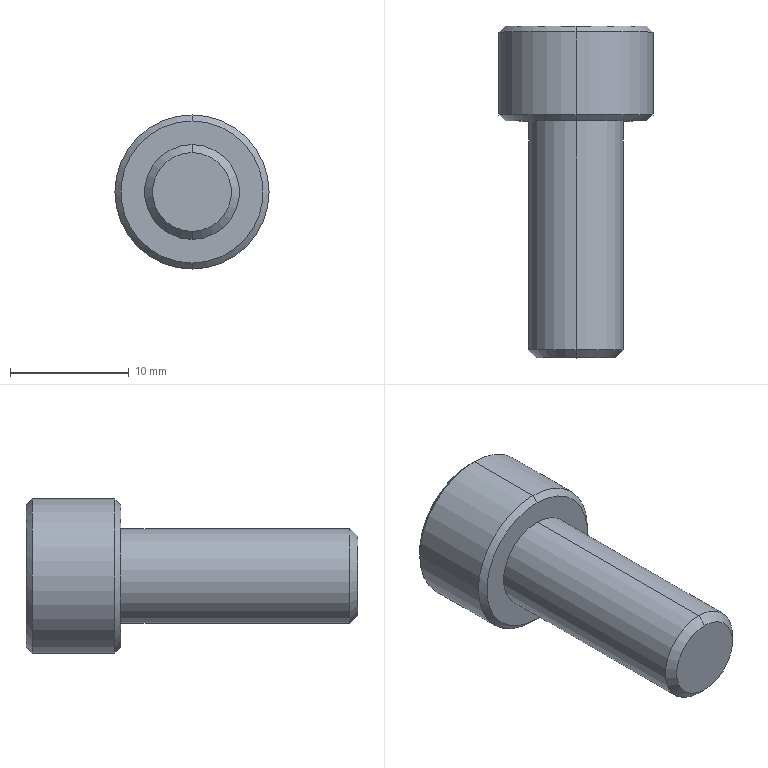Part | SolidWorks | features ICE 2, Chamfer 1, Extrusion 1, StudWizard 1 | 1 solid | 20 faces | box 13 x 28 x 13 mm | volume 1927 mm3 | plane 10 | cone 6 | cylinder 4 | commonest cylinder face diameters 8 x2 13 x2
STEP:
#1=CARTESIAN_POINT('',(0.,0.,3.324));
#2=VERTEX_POINT('',#1);
#3=CARTESIAN_POINT('',(0.,0.,-3.324));
#4=VERTEX_POINT('',#3);
#5=CARTESIAN_POINT('',(0.,0.,0.));
#6=DIRECTION('',(0.,1.,0.));
#7=DIRECTION('',(0.,0.,1.));
#8=AXIS2_PLACEMENT_3D('',#5,#6,#7);
#9=CIRCLE('',#8,3.324);
#10=EDGE_CURVE('',#2,#4,#9,.T.);
#11=ORIENTED_EDGE('',*,*,#10,.T.);
#12=CARTESIAN_POINT('',(0.,0.6765,-4.));
#13=VERTEX_POINT('',#12);
#14=CARTESIAN_POINT('',(0.,0.,-3.324));
#15=DIRECTION('',(0.,0.7071,-0.7071));
#16=VECTOR('',#15,1000.);
#17=LINE('',#14,#16);
#18=EDGE_CURVE('',#4,#13,#17,.T.);
#19=ORIENTED_EDGE('',*,*,#18,.T.);
#20=CARTESIAN_POINT('',(0.,0.6765,4.));
#21=VERTEX_POINT('',#20);
#22=CARTESIAN_POINT('',(0.,0.6765,0.));
#23=DIRECTION('',(0.,1.,0.));
#24=DIRECTION('',(0.,0.,1.));
#25=AXIS2_PLACEMENT_3D('',#22,#23,#24);
#26=CIRCLE('',#25,4.);
#27=EDGE_CURVE('',#21,#13,#26,.T.);
#28=ORIENTED_EDGE('',*,*,#27,.F.);
#29=CARTESIAN_POINT('',(0.,0.,3.324));
#30=DIRECTION('',(0.,0.7071,0.7071));
#31=VECTOR('',#30,1000.);
#32=LINE('',#29,#31);
#33=EDGE_CURVE('',#2,#21,#32,.T.);
#34=ORIENTED_EDGE('',*,*,#33,.F.);
#35=EDGE_LOOP('',(#11,#19,#28,#34));
#36=FACE_OUTER_BOUND('',#35,.T.);
#37=CARTESIAN_POINT('',(0.,0.,0.));
#38=DIRECTION('',(0.,1.,0.));
#39=DIRECTION('',(0.,0.,1.));
#40=AXIS2_PLACEMENT_3D('',#37,#38,#39);
#41=CONICAL_SURFACE('',#40,3.324,0.7854);
#42=ADVANCED_FACE('',(#36),#41,.T.);
#43=CARTESIAN_POINT('',(0.,28.,6.));
#44=VERTEX_POINT('',#43);
#45=CARTESIAN_POINT('',(0.,28.,-6.));
#46=VERTEX_POINT('',#45);
#47=CARTESIAN_POINT('',(0.,28.,0.));
#48=DIRECTION('',(0.,1.,0.));
#49=DIRECTION('',(0.,0.,1.));
#50=AXIS2_PLACEMENT_3D('',#47,#48,#49);
#51=CIRCLE('',#50,6.);
#52=EDGE_CURVE('',#44,#46,#51,.T.);
#53=ORIENTED_EDGE('',*,*,#52,.F.);
#54=CARTESIAN_POINT('',(0.,27.5,6.5));
#55=VERTEX_POINT('',#54);
#56=CARTESIAN_POINT('',(0.,28.,6.));
#57=DIRECTION('',(0.,-0.7071,0.7071));
#58=VECTOR('',#57,1000.);
#59=LINE('',#56,#58);
#60=EDGE_CURVE('',#44,#55,#59,.T.);
#61=ORIENTED_EDGE('',*,*,#60,.T.);
#62=CARTESIAN_POINT('',(0.,27.5,-6.5));
#63=VERTEX_POINT('',#62);
#64=CARTESIAN_POINT('',(0.,27.5,0.));
#65=DIRECTION('',(0.,-1.,0.));
#66=DIRECTION('',(0.,0.,1.));
#67=AXIS2_PLACEMENT_3D('',#64,#65,#66);
#68=CIRCLE('',#67,6.5);
#69=EDGE_CURVE('',#63,#55,#68,.T.);
#70=ORIENTED_EDGE('',*,*,#69,.F.);
#71=CARTESIAN_POINT('',(0.,28.,-6.));
#72=DIRECTION('',(0.,-0.7071,-0.7071));
#73=VECTOR('',#72,1000.);
#74=LINE('',#71,#73);
#75=EDGE_CURVE('',#46,#63,#74,.T.);
#76=ORIENTED_EDGE('',*,*,#75,.F.);
#77=EDGE_LOOP('',(#53,#61,#70,#76));
#78=FACE_OUTER_BOUND('',#77,.T.);
#79=CARTESIAN_POINT('',(0.,28.,0.));
#80=DIRECTION('',(0.,-1.,0.));
#81=DIRECTION('',(0.,0.,-1.));
#82=AXIS2_PLACEMENT_3D('',#79,#80,#81);
#83=CONICAL_SURFACE('',#82,6.,0.7854);
#84=ADVANCED_FACE('',(#78),#83,.T.);
#85=CARTESIAN_POINT('',(0.,20.,-6.));
#86=VERTEX_POINT('',#85);
#87=CARTESIAN_POINT('',(0.,20.,6.));
#88=VERTEX_POINT('',#87);
#89=CARTESIAN_POINT('',(0.,20.,0.));
#90=DIRECTION('',(0.,-1.,0.));
#91=DIRECTION('',(0.,0.,1.));
#92=AXIS2_PLACEMENT_3D('',#89,#90,#91);
#93=CIRCLE('',#92,6.);
#94=EDGE_CURVE('',#86,#88,#93,.T.);
#95=ORIENTED_EDGE('',*,*,#94,.F.);
#96=CARTESIAN_POINT('',(0.,20.5,-6.5));
#97=VERTEX_POINT('',#96);
#98=CARTESIAN_POINT('',(0.,20.5,-6.5));
#99=DIRECTION('',(0.,0.7071,-0.7071));
#100=VECTOR('',#99,1000.);
#101=LINE('',#98,#100);
#102=EDGE_CURVE('',#86,#97,#101,.T.);
#103=ORIENTED_EDGE('',*,*,#102,.T.);
#104=CARTESIAN_POINT('',(0.,20.5,6.5));
#105=VERTEX_POINT('',#104);
#106=CARTESIAN_POINT('',(0.,20.5,0.));
#107=DIRECTION('',(0.,1.,0.));
#108=DIRECTION('',(0.,0.,1.));
#109=AXIS2_PLACEMENT_3D('',#106,#107,#108);
#110=CIRCLE('',#109,6.5);
#111=EDGE_CURVE('',#105,#97,#110,.T.);
#112=ORIENTED_EDGE('',*,*,#111,.F.);
#113=CARTESIAN_POINT('',(0.,20.5,6.5));
#114=DIRECTION('',(0.,0.7071,0.7071));
#115=VECTOR('',#114,1000.);
#116=LINE('',#113,#115);
#117=EDGE_CURVE('',#88,#105,#116,.T.);
#118=ORIENTED_EDGE('',*,*,#117,.F.);
#119=EDGE_LOOP('',(#95,#103,#112,#118));
#120=FACE_OUTER_BOUND('',#119,.T.);
#121=CARTESIAN_POINT('',(0.,20.5,0.));
#122=DIRECTION('',(0.,1.,0.));
#123=DIRECTION('',(0.,0.,1.));
#124=AXIS2_PLACEMENT_3D('',#121,#122,#123);
#125=CONICAL_SURFACE('',#124,6.5,0.7854);
#126=ADVANCED_FACE('',(#120),#125,.T.);
#127=ORIENTED_EDGE('',*,*,#69,.T.);
#128=CARTESIAN_POINT('',(0.,28.,6.5));
#129=DIRECTION('',(0.,-1.,0.));
#130=VECTOR('',#129,1000.);
#131=LINE('',#128,#130);
#132=EDGE_CURVE('',#55,#105,#131,.T.);
#133=ORIENTED_EDGE('',*,*,#132,.T.);
#134=ORIENTED_EDGE('',*,*,#111,.T.);
#135=CARTESIAN_POINT('',(0.,28.,-6.5));
#136=DIRECTION('',(0.,-1.,0.));
#137=VECTOR('',#136,1000.);
#138=LINE('',#135,#137);
#139=EDGE_CURVE('',#63,#97,#138,.T.);
#140=ORIENTED_EDGE('',*,*,#139,.F.);
#141=EDGE_LOOP('',(#127,#133,#134,#140));
#142=FACE_OUTER_BOUND('',#141,.T.);
#143=CARTESIAN_POINT('',(0.,28.,0.));
#144=DIRECTION('',(0.,-1.,0.));
#145=DIRECTION('',(0.,0.,-1.));
#146=AXIS2_PLACEMENT_3D('',#143,#144,#145);
#147=CYLINDRICAL_SURFACE('',#146,6.5);
#148=ADVANCED_FACE('',(#142),#147,.T.);
#149=CARTESIAN_POINT('',(0.,20.,4.));
#150=VERTEX_POINT('',#149);
#151=CARTESIAN_POINT('',(0.,20.,-4.));
#152=VERTEX_POINT('',#151);
#153=CARTESIAN_POINT('',(0.,20.,0.));
#154=DIRECTION('',(0.,1.,0.));
#155=DIRECTION('',(0.,0.,1.));
#156=AXIS2_PLACEMENT_3D('',#153,#154,#155);
#157=CIRCLE('',#156,4.);
#158=EDGE_CURVE('',#150,#152,#157,.T.);
#159=ORIENTED_EDGE('',*,*,#158,.F.);
#160=CARTESIAN_POINT('',(0.,20.,4.));
#161=DIRECTION('',(0.,-1.,0.));
#162=VECTOR('',#161,1000.);
#163=LINE('',#160,#162);
#164=EDGE_CURVE('',#150,#21,#163,.T.);
#165=ORIENTED_EDGE('',*,*,#164,.T.);
#166=ORIENTED_EDGE('',*,*,#27,.T.);
#167=CARTESIAN_POINT('',(0.,20.,-4.));
#168=DIRECTION('',(0.,-1.,0.));
#169=VECTOR('',#168,1000.);
#170=LINE('',#167,#169);
#171=EDGE_CURVE('',#152,#13,#170,.T.);
#172=ORIENTED_EDGE('',*,*,#171,.F.);
#173=EDGE_LOOP('',(#159,#165,#166,#172));
#174=FACE_OUTER_BOUND('',#173,.T.);
#175=CARTESIAN_POINT('',(0.,20.,0.));
#176=DIRECTION('',(0.,-1.,0.));
#177=DIRECTION('',(0.,0.,-1.));
#178=AXIS2_PLACEMENT_3D('',#175,#176,#177);
#179=CYLINDRICAL_SURFACE('',#178,4.);
#180=ADVANCED_FACE('',(#174),#179,.T.);
#181=ORIENTED_EDGE('',*,*,#164,.F.);
#182=CARTESIAN_POINT('',(0.,20.,0.));
#183=DIRECTION('',(0.,1.,0.));
#184=DIRECTION('',(0.,0.,1.));
#185=AXIS2_PLACEMENT_3D('',#182,#183,#184);
#186=CIRCLE('',#185,4.);
#187=EDGE_CURVE('',#152,#150,#186,.T.);
#188=ORIENTED_EDGE('',*,*,#187,.F.);
#189=ORIENTED_EDGE('',*,*,#171,.T.);
#190=CARTESIAN_POINT('',(0.,0.6765,0.));
#191=DIRECTION('',(0.,1.,0.));
#192=DIRECTION('',(0.,0.,1.));
#193=AXIS2_PLACEMENT_3D('',#190,#191,#192);
#194=CIRCLE('',#193,4.);
#195=EDGE_CURVE('',#13,#21,#194,.T.);
#196=ORIENTED_EDGE('',*,*,#195,.T.);
#197=EDGE_LOOP('',(#181,#188,#189,#196));
#198=FACE_OUTER_BOUND('',#197,.T.);
#199=CARTESIAN_POINT('',(0.,20.,0.));
#200=DIRECTION('',(0.,-1.,0.));
#201=DIRECTION('',(0.,0.,-1.));
#202=AXIS2_PLACEMENT_3D('',#199,#200,#201);
#203=CYLINDRICAL_SURFACE('',#202,4.);
#204=ADVANCED_FACE('',(#198),#203,.T.);
#205=ORIENTED_EDGE('',*,*,#132,.F.);
#206=CARTESIAN_POINT('',(0.,27.5,0.));
#207=DIRECTION('',(0.,-1.,0.));
#208=DIRECTION('',(0.,0.,1.));
#209=AXIS2_PLACEMENT_3D('',#206,#207,#208);
#210=CIRCLE('',#209,6.5);
#211=EDGE_CURVE('',#55,#63,#210,.T.);
#212=ORIENTED_EDGE('',*,*,#211,.T.);
#213=ORIENTED_EDGE('',*,*,#139,.T.);
#214=CARTESIAN_POINT('',(0.,20.5,0.));
#215=DIRECTION('',(0.,1.,0.));
#216=DIRECTION('',(0.,0.,1.));
#217=AXIS2_PLACEMENT_3D('',#214,#215,#216);
#218=CIRCLE('',#217,6.5);
#219=EDGE_CURVE('',#97,#105,#218,.T.);
#220=ORIENTED_EDGE('',*,*,#219,.T.);
#221=EDGE_LOOP('',(#205,#212,#213,#220));
#222=FACE_OUTER_BOUND('',#221,.T.);
#223=CARTESIAN_POINT('',(0.,28.,0.));
#224=DIRECTION('',(0.,-1.,0.));
#225=DIRECTION('',(0.,0.,-1.));
#226=AXIS2_PLACEMENT_3D('',#223,#224,#225);
#227=CYLINDRICAL_SURFACE('',#226,6.5);
#228=ADVANCED_FACE('',(#222),#227,.T.);
#229=CARTESIAN_POINT('',(0.,28.,0.));
#230=DIRECTION('',(0.,1.,0.));
#231=DIRECTION('',(0.,0.,1.));
#232=AXIS2_PLACEMENT_3D('',#229,#230,#231);
#233=CIRCLE('',#232,6.);
#234=EDGE_CURVE('',#46,#44,#233,.T.);
#235=ORIENTED_EDGE('',*,*,#234,.T.);
#236=ORIENTED_EDGE('',*,*,#52,.T.);
#237=EDGE_LOOP('',(#235,#236));
#238=FACE_OUTER_BOUND('',#237,.T.);
#239=CARTESIAN_POINT('',(3.,28.,-1.732));
#240=VERTEX_POINT('',#239);
#241=CARTESIAN_POINT('',(0.,28.,-3.464));
#242=VERTEX_POINT('',#241);
#243=CARTESIAN_POINT('',(3.,28.,-1.732));
#244=DIRECTION('',(-0.866,0.,-0.5));
#245=VECTOR('',#244,1000.);
#246=LINE('',#243,#245);
#247=EDGE_CURVE('',#240,#242,#246,.T.);
#248=ORIENTED_EDGE('',*,*,#247,.F.);
#249=CARTESIAN_POINT('',(3.,28.,1.732));
#250=VERTEX_POINT('',#249);
#251=CARTESIAN_POINT('',(3.,28.,1.732));
#252=DIRECTION('',(0.,0.,-1.));
#253=VECTOR('',#252,1000.);
#254=LINE('',#251,#253);
#255=EDGE_CURVE('',#250,#240,#254,.T.);
#256=ORIENTED_EDGE('',*,*,#255,.F.);
#257=CARTESIAN_POINT('',(0.,28.,3.464));
#258=VERTEX_POINT('',#257);
#259=CARTESIAN_POINT('',(0.,28.,3.464));
#260=DIRECTION('',(0.866,0.,-0.5));
#261=VECTOR('',#260,1000.);
#262=LINE('',#259,#261);
#263=EDGE_CURVE('',#258,#250,#262,.T.);
#264=ORIENTED_EDGE('',*,*,#263,.F.);
#265=CARTESIAN_POINT('',(-3.,28.,1.732));
#266=VERTEX_POINT('',#265);
#267=CARTESIAN_POINT('',(-3.,28.,1.732));
#268=DIRECTION('',(0.866,0.,0.5));
#269=VECTOR('',#268,1000.);
#270=LINE('',#267,#269);
#271=EDGE_CURVE('',#266,#258,#270,.T.);
#272=ORIENTED_EDGE('',*,*,#271,.F.);
#273=CARTESIAN_POINT('',(-3.,28.,-1.732));
#274=VERTEX_POINT('',#273);
#275=CARTESIAN_POINT('',(-3.,28.,-1.732));
#276=DIRECTION('',(0.,0.,1.));
#277=VECTOR('',#276,1000.);
#278=LINE('',#275,#277);
#279=EDGE_CURVE('',#274,#266,#278,.T.);
#280=ORIENTED_EDGE('',*,*,#279,.F.);
#281=CARTESIAN_POINT('',(0.,28.,-3.464));
#282=DIRECTION('',(-0.866,0.,0.5));
#283=VECTOR('',#282,1000.);
#284=LINE('',#281,#283);
#285=EDGE_CURVE('',#242,#274,#284,.T.);
#286=ORIENTED_EDGE('',*,*,#285,.F.);
#287=EDGE_LOOP('',(#248,#256,#264,#272,#280,#286));
#288=FACE_BOUND('',#287,.T.);
#289=CARTESIAN_POINT('',(0.,28.,0.));
#290=DIRECTION('',(0.,1.,0.));
#291=DIRECTION('',(0.,0.,1.));
#292=AXIS2_PLACEMENT_3D('',#289,#290,#291);
#293=PLANE('',#292);
#294=ADVANCED_FACE('',(#238,#288),#293,.T.);
#295=CARTESIAN_POINT('',(0.,20.,0.));
#296=DIRECTION('',(0.,-1.,0.));
#297=DIRECTION('',(0.,0.,1.));
#298=AXIS2_PLACEMENT_3D('',#295,#296,#297);
#299=CIRCLE('',#298,6.);
#300=EDGE_CURVE('',#88,#86,#299,.T.);
#301=ORIENTED_EDGE('',*,*,#300,.T.);
#302=ORIENTED_EDGE('',*,*,#94,.T.);
#303=EDGE_LOOP('',(#301,#302));
#304=FACE_OUTER_BOUND('',#303,.T.);
#305=ORIENTED_EDGE('',*,*,#187,.T.);
#306=ORIENTED_EDGE('',*,*,#158,.T.);
#307=EDGE_LOOP('',(#305,#306));
#308=FACE_BOUND('',#307,.T.);
#309=CARTESIAN_POINT('',(0.,20.,0.));
#310=DIRECTION('',(0.,1.,0.));
#311=DIRECTION('',(0.,0.,1.));
#312=AXIS2_PLACEMENT_3D('',#309,#310,#311);
#313=PLANE('',#312);
#314=ADVANCED_FACE('',(#304,#308),#313,.F.);
#315=ORIENTED_EDGE('',*,*,#247,.T.);
#316=CARTESIAN_POINT('',(0.,24.,-3.464));
#317=VERTEX_POINT('',#316);
#318=CARTESIAN_POINT('',(0.,24.,-3.464));
#319=DIRECTION('',(0.,1.,0.));
#320=VECTOR('',#319,1000.);
#321=LINE('',#318,#320);
#322=EDGE_CURVE('',#317,#242,#321,.T.);
#323=ORIENTED_EDGE('',*,*,#322,.F.);
#324=CARTESIAN_POINT('',(3.,24.,-1.732));
#325=VERTEX_POINT('',#324);
#326=CARTESIAN_POINT('',(3.,24.,-1.732));
#327=DIRECTION('',(-0.866,0.,-0.5));
#328=VECTOR('',#327,1000.);
#329=LINE('',#326,#328);
#330=EDGE_CURVE('',#325,#317,#329,.T.);
#331=ORIENTED_EDGE('',*,*,#330,.F.);
#332=CARTESIAN_POINT('',(3.,24.,-1.732));
#333=DIRECTION('',(0.,1.,0.));
#334=VECTOR('',#333,1000.);
#335=LINE('',#332,#334);
#336=EDGE_CURVE('',#325,#240,#335,.T.);
#337=ORIENTED_EDGE('',*,*,#336,.T.);
#338=EDGE_LOOP('',(#315,#323,#331,#337));
#339=FACE_OUTER_BOUND('',#338,.T.);
#340=CARTESIAN_POINT('',(3.,24.,-1.732));
#341=DIRECTION('',(0.5,0.,-0.866));
#342=DIRECTION('',(-0.866,0.,-0.5));
#343=AXIS2_PLACEMENT_3D('',#340,#341,#342);
#344=PLANE('',#343);
#345=ADVANCED_FACE('',(#339),#344,.F.);
#346=ORIENTED_EDGE('',*,*,#255,.T.);
#347=ORIENTED_EDGE('',*,*,#336,.F.);
#348=CARTESIAN_POINT('',(3.,24.,1.732));
#349=VERTEX_POINT('',#348);
#350=CARTESIAN_POINT('',(3.,24.,1.732));
#351=DIRECTION('',(0.,0.,-1.));
#352=VECTOR('',#351,1000.);
#353=LINE('',#350,#352);
#354=EDGE_CURVE('',#349,#325,#353,.T.);
#355=ORIENTED_EDGE('',*,*,#354,.F.);
#356=CARTESIAN_POINT('',(3.,24.,1.732));
#357=DIRECTION('',(0.,1.,0.));
#358=VECTOR('',#357,1000.);
#359=LINE('',#356,#358);
#360=EDGE_CURVE('',#349,#250,#359,.T.);
#361=ORIENTED_EDGE('',*,*,#360,.T.);
#362=EDGE_LOOP('',(#346,#347,#355,#361));
#363=FACE_OUTER_BOUND('',#362,.T.);
#364=CARTESIAN_POINT('',(3.,24.,1.732));
#365=DIRECTION('',(1.,0.,0.));
#366=DIRECTION('',(0.,0.,-1.));
#367=AXIS2_PLACEMENT_3D('',#364,#365,#366);
#368=PLANE('',#367);
#369=ADVANCED_FACE('',(#363),#368,.F.);
#370=ORIENTED_EDGE('',*,*,#263,.T.);
#371=ORIENTED_EDGE('',*,*,#360,.F.);
#372=CARTESIAN_POINT('',(0.,24.,3.464));
#373=VERTEX_POINT('',#372);
#374=CARTESIAN_POINT('',(0.,24.,3.464));
#375=DIRECTION('',(0.866,0.,-0.5));
#376=VECTOR('',#375,1000.);
#377=LINE('',#374,#376);
#378=EDGE_CURVE('',#373,#349,#377,.T.);
#379=ORIENTED_EDGE('',*,*,#378,.F.);
#380=CARTESIAN_POINT('',(0.,24.,3.464));
#381=DIRECTION('',(0.,1.,0.));
#382=VECTOR('',#381,1000.);
#383=LINE('',#380,#382);
#384=EDGE_CURVE('',#373,#258,#383,.T.);
#385=ORIENTED_EDGE('',*,*,#384,.T.);
#386=EDGE_LOOP('',(#370,#371,#379,#385));
#387=FACE_OUTER_BOUND('',#386,.T.);
#388=CARTESIAN_POINT('',(0.,24.,3.464));
#389=DIRECTION('',(0.5,0.,0.866));
#390=DIRECTION('',(0.866,0.,-0.5));
#391=AXIS2_PLACEMENT_3D('',#388,#389,#390);
#392=PLANE('',#391);
#393=ADVANCED_FACE('',(#387),#392,.F.);
#394=ORIENTED_EDGE('',*,*,#271,.T.);
#395=ORIENTED_EDGE('',*,*,#384,.F.);
#396=CARTESIAN_POINT('',(-3.,24.,1.732));
#397=VERTEX_POINT('',#396);
#398=CARTESIAN_POINT('',(-3.,24.,1.732));
#399=DIRECTION('',(0.866,0.,0.5));
#400=VECTOR('',#399,1000.);
#401=LINE('',#398,#400);
#402=EDGE_CURVE('',#397,#373,#401,.T.);
#403=ORIENTED_EDGE('',*,*,#402,.F.);
#404=CARTESIAN_POINT('',(-3.,24.,1.732));
#405=DIRECTION('',(0.,1.,0.));
#406=VECTOR('',#405,1000.);
#407=LINE('',#404,#406);
#408=EDGE_CURVE('',#397,#266,#407,.T.);
#409=ORIENTED_EDGE('',*,*,#408,.T.);
#410=EDGE_LOOP('',(#394,#395,#403,#409));
#411=FACE_OUTER_BOUND('',#410,.T.);
#412=CARTESIAN_POINT('',(-3.,24.,1.732));
#413=DIRECTION('',(-0.5,0.,0.866));
#414=DIRECTION('',(0.866,0.,0.5));
#415=AXIS2_PLACEMENT_3D('',#412,#413,#414);
#416=PLANE('',#415);
#417=ADVANCED_FACE('',(#411),#416,.F.);
#418=ORIENTED_EDGE('',*,*,#279,.T.);
#419=ORIENTED_EDGE('',*,*,#408,.F.);
#420=CARTESIAN_POINT('',(-3.,24.,-1.732));
#421=VERTEX_POINT('',#420);
#422=CARTESIAN_POINT('',(-3.,24.,-1.732));
#423=DIRECTION('',(0.,0.,1.));
#424=VECTOR('',#423,1000.);
#425=LINE('',#422,#424);
#426=EDGE_CURVE('',#421,#397,#425,.T.);
#427=ORIENTED_EDGE('',*,*,#426,.F.);
#428=CARTESIAN_POINT('',(-3.,24.,-1.732));
#429=DIRECTION('',(0.,1.,0.));
#430=VECTOR('',#429,1000.);
#431=LINE('',#428,#430);
#432=EDGE_CURVE('',#421,#274,#431,.T.);
#433=ORIENTED_EDGE('',*,*,#432,.T.);
#434=EDGE_LOOP('',(#418,#419,#427,#433));
#435=FACE_OUTER_BOUND('',#434,.T.);
#436=CARTESIAN_POINT('',(-3.,24.,-1.732));
#437=DIRECTION('',(-1.,0.,0.));
#438=DIRECTION('',(0.,0.,1.));
#439=AXIS2_PLACEMENT_3D('',#436,#437,#438);
#440=PLANE('',#439);
#441=ADVANCED_FACE('',(#435),#440,.F.);
#442=ORIENTED_EDGE('',*,*,#285,.T.);
#443=ORIENTED_EDGE('',*,*,#432,.F.);
#444=CARTESIAN_POINT('',(0.,24.,-3.464));
#445=DIRECTION('',(-0.866,0.,0.5));
#446=VECTOR('',#445,1000.);
#447=LINE('',#444,#446);
#448=EDGE_CURVE('',#317,#421,#447,.T.);
#449=ORIENTED_EDGE('',*,*,#448,.F.);
#450=ORIENTED_EDGE('',*,*,#322,.T.);
#451=EDGE_LOOP('',(#442,#443,#449,#450));
#452=FACE_OUTER_BOUND('',#451,.T.);
#453=CARTESIAN_POINT('',(0.,24.,-3.464));
#454=DIRECTION('',(-0.5,0.,-0.866));
#455=DIRECTION('',(-0.866,0.,0.5));
#456=AXIS2_PLACEMENT_3D('',#453,#454,#455);
#457=PLANE('',#456);
#458=ADVANCED_FACE('',(#452),#457,.F.);
#459=ORIENTED_EDGE('',*,*,#330,.T.);
#460=ORIENTED_EDGE('',*,*,#448,.T.);
#461=ORIENTED_EDGE('',*,*,#426,.T.);
#462=ORIENTED_EDGE('',*,*,#402,.T.);
#463=ORIENTED_EDGE('',*,*,#378,.T.);
#464=ORIENTED_EDGE('',*,*,#354,.T.);
#465=EDGE_LOOP('',(#459,#460,#461,#462,#463,#464));
#466=FACE_OUTER_BOUND('',#465,.T.);
#467=CARTESIAN_POINT('',(0.,24.,0.));
#468=DIRECTION('',(0.,1.,0.));
#469=DIRECTION('',(0.,0.,1.));
#470=AXIS2_PLACEMENT_3D('',#467,#468,#469);
#471=PLANE('',#470);
#472=ADVANCED_FACE('',(#466),#471,.T.);
#473=ORIENTED_EDGE('',*,*,#102,.F.);
#474=ORIENTED_EDGE('',*,*,#300,.F.);
#475=ORIENTED_EDGE('',*,*,#117,.T.);
#476=ORIENTED_EDGE('',*,*,#219,.F.);
#477=EDGE_LOOP('',(#473,#474,#475,#476));
#478=FACE_OUTER_BOUND('',#477,.T.);
#479=CARTESIAN_POINT('',(0.,20.5,0.));
#480=DIRECTION('',(0.,1.,0.));
#481=DIRECTION('',(0.,0.,1.));
#482=AXIS2_PLACEMENT_3D('',#479,#480,#481);
#483=CONICAL_SURFACE('',#482,6.5,0.7854);
#484=ADVANCED_FACE('',(#478),#483,.T.);
#485=ORIENTED_EDGE('',*,*,#60,.F.);
#486=ORIENTED_EDGE('',*,*,#234,.F.);
#487=ORIENTED_EDGE('',*,*,#75,.T.);
#488=ORIENTED_EDGE('',*,*,#211,.F.);
#489=EDGE_LOOP('',(#485,#486,#487,#488));
#490=FACE_OUTER_BOUND('',#489,.T.);
#491=CARTESIAN_POINT('',(0.,28.,0.));
#492=DIRECTION('',(0.,-1.,0.));
#493=DIRECTION('',(0.,0.,-1.));
#494=AXIS2_PLACEMENT_3D('',#491,#492,#493);
#495=CONICAL_SURFACE('',#494,6.,0.7854);
#496=ADVANCED_FACE('',(#490),#495,.T.);
#497=ORIENTED_EDGE('',*,*,#18,.F.);
#498=CARTESIAN_POINT('',(0.,0.,0.));
#499=DIRECTION('',(0.,1.,0.));
#500=DIRECTION('',(0.,0.,1.));
#501=AXIS2_PLACEMENT_3D('',#498,#499,#500);
#502=CIRCLE('',#501,3.324);
#503=EDGE_CURVE('',#4,#2,#502,.T.);
#504=ORIENTED_EDGE('',*,*,#503,.T.);
#505=ORIENTED_EDGE('',*,*,#33,.T.);
#506=ORIENTED_EDGE('',*,*,#195,.F.);
#507=EDGE_LOOP('',(#497,#504,#505,#506));
#508=FACE_OUTER_BOUND('',#507,.T.);
#509=CARTESIAN_POINT('',(0.,0.,0.));
#510=DIRECTION('',(0.,1.,0.));
#511=DIRECTION('',(0.,0.,1.));
#512=AXIS2_PLACEMENT_3D('',#509,#510,#511);
#513=CONICAL_SURFACE('',#512,3.324,0.7854);
#514=ADVANCED_FACE('',(#508),#513,.T.);
#515=ORIENTED_EDGE('',*,*,#10,.F.);
#516=ORIENTED_EDGE('',*,*,#503,.F.);
#517=EDGE_LOOP('',(#515,#516));
#518=FACE_OUTER_BOUND('',#517,.T.);
#519=CARTESIAN_POINT('',(0.,0.,0.));
#520=DIRECTION('',(0.,1.,0.));
#521=DIRECTION('',(0.,0.,1.));
#522=AXIS2_PLACEMENT_3D('',#519,#520,#521);
#523=PLANE('',#522);
#524=ADVANCED_FACE('',(#518),#523,.F.);
#525=CLOSED_SHELL('',(#42,#84,#126,#148,#180,#204,#228,#294,#314,#345,#369,#393,#417,#441,#458,#472,#484,#496,#514,#524));
#526=MANIFOLD_SOLID_BREP('',#525);
#527=CARTESIAN_POINT('',(0.,0.,0.));
#528=DIRECTION('',(0.,0.,1.));
#529=DIRECTION('',(1.,0.,0.));
#530=AXIS2_PLACEMENT_3D('',#527,#528,#529);
#531=(LENGTH_UNIT()NAMED_UNIT(*)SI_UNIT(.MILLI.,.METRE.));
#532=UNCERTAINTY_MEASURE_WITH_UNIT(LENGTH_MEASURE(0.00001),#531,'','');
#533=(NAMED_UNIT(*)PLANE_ANGLE_UNIT()SI_UNIT($,.RADIAN.));
#534=(NAMED_UNIT(*)SI_UNIT($,.STERADIAN.)SOLID_ANGLE_UNIT());
#535=(GEOMETRIC_REPRESENTATION_CONTEXT(3)GLOBAL_UNCERTAINTY_ASSIGNED_CONTEXT((#532))GLOBAL_UNIT_ASSIGNED_CONTEXT((#531,#533,#534))REPRESENTATION_CONTEXT('',''));
#536=ADVANCED_BREP_SHAPE_REPRESENTATION('',(#526,#530),#535);